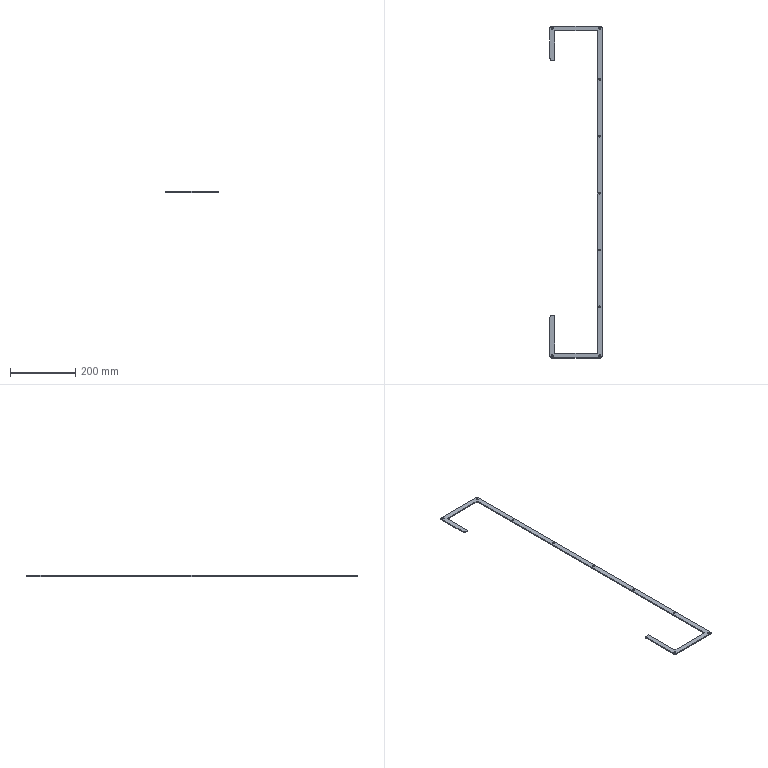Part | STEP file | Input 82 | 1 solid | 38 faces | box 160 x 1020 x 3.2 mm | volume 71803 mm3 | cylinder 24 | plane 14 | commonest cylinder face diameters 6 x18 10 x6